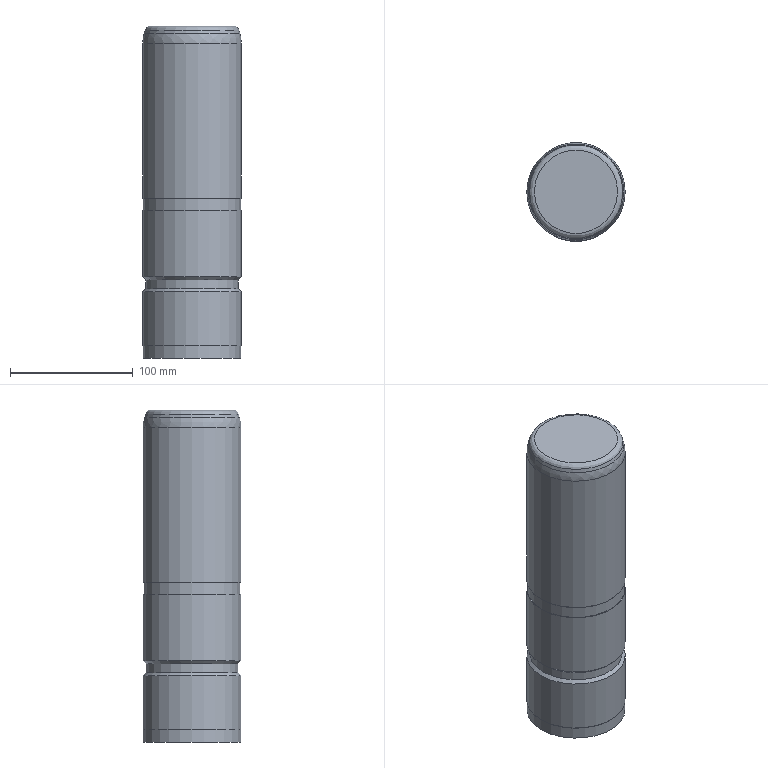Part | NX | features solid 2 | 1 solid | 16 faces | box 80 x 80 x 270 mm | volume 1345505 mm3 | cylinder 6 | plane 5 | cone 3 | torus 2 | commonest cylinder face diameters 80 x3 75 x1 79 x1 79.5 x1
STEP:
#1=CARTESIAN_POINT('',(-1152.5,955.,-291.5));
#2=VERTEX_POINT('',#1);
#3=CARTESIAN_POINT('',(-1115.,955.,-291.5));
#4=DIRECTION('',(0.,0.,1.));
#5=DIRECTION('',(-1.,0.,0.));
#6=AXIS2_PLACEMENT_3D('',#3,#4,#5);
#7=CIRCLE('',#6,37.5);
#8=EDGE_CURVE('',#2,#2,#7,.T.);
#9=ORIENTED_EDGE('',*,*,#8,.T.);
#10=EDGE_LOOP('',(#9));
#11=FACE_BOUND('',#10,.T.);
#12=CARTESIAN_POINT('',(-1075.,955.,-289.));
#13=VERTEX_POINT('',#12);
#14=CARTESIAN_POINT('',(-1115.,955.,-289.));
#15=DIRECTION('',(0.,0.,-1.));
#16=DIRECTION('',(1.,0.,0.));
#17=AXIS2_PLACEMENT_3D('',#14,#15,#16);
#18=CIRCLE('',#17,40.);
#19=EDGE_CURVE('',#13,#13,#18,.T.);
#20=ORIENTED_EDGE('',*,*,#19,.T.);
#21=EDGE_LOOP('',(#20));
#22=FACE_BOUND('',#21,.T.);
#23=CARTESIAN_POINT('',(-1115.,955.,-291.5));
#24=DIRECTION('',(0.,0.,1.));
#25=DIRECTION('',(1.,0.,0.));
#26=AXIS2_PLACEMENT_3D('',#23,#24,#25);
#27=CONICAL_SURFACE('',#26,37.5,0.7854);
#28=ADVANCED_FACE('',(#11,#22),#27,.T.);
#29=ORIENTED_EDGE('',*,*,#8,.F.);
#30=EDGE_LOOP('',(#29));
#31=FACE_BOUND('',#30,.T.);
#32=CARTESIAN_POINT('',(-1152.5,955.,-298.5));
#33=VERTEX_POINT('',#32);
#34=CARTESIAN_POINT('',(-1115.,955.,-298.5));
#35=DIRECTION('',(0.,0.,1.));
#36=DIRECTION('',(-1.,0.,0.));
#37=AXIS2_PLACEMENT_3D('',#34,#35,#36);
#38=CIRCLE('',#37,37.5);
#39=EDGE_CURVE('',#33,#33,#38,.T.);
#40=ORIENTED_EDGE('',*,*,#39,.T.);
#41=EDGE_LOOP('',(#40));
#42=FACE_BOUND('',#41,.T.);
#43=CARTESIAN_POINT('',(-1115.,955.,-298.5));
#44=DIRECTION('',(0.,0.,1.));
#45=DIRECTION('',(1.,0.,0.));
#46=AXIS2_PLACEMENT_3D('',#43,#44,#45);
#47=CYLINDRICAL_SURFACE('',#46,37.5);
#48=ADVANCED_FACE('',(#31,#42),#47,.T.);
#49=CARTESIAN_POINT('',(-1075.5,955.,-235.));
#50=VERTEX_POINT('',#49);
#51=CARTESIAN_POINT('',(-1115.,955.,-235.));
#52=DIRECTION('',(0.,0.,-1.));
#53=DIRECTION('',(1.,0.,0.));
#54=AXIS2_PLACEMENT_3D('',#51,#52,#53);
#55=CIRCLE('',#54,39.5);
#56=EDGE_CURVE('',#50,#50,#55,.T.);
#57=ORIENTED_EDGE('',*,*,#56,.T.);
#58=EDGE_LOOP('',(#57));
#59=FACE_BOUND('',#58,.T.);
#60=CARTESIAN_POINT('',(-1155.,955.,-235.));
#61=VERTEX_POINT('',#60);
#62=CARTESIAN_POINT('',(-1115.,955.,-235.));
#63=DIRECTION('',(0.,0.,1.));
#64=DIRECTION('',(-1.,0.,0.));
#65=AXIS2_PLACEMENT_3D('',#62,#63,#64);
#66=CIRCLE('',#65,40.);
#67=EDGE_CURVE('',#61,#61,#66,.T.);
#68=ORIENTED_EDGE('',*,*,#67,.T.);
#69=EDGE_LOOP('',(#68));
#70=FACE_BOUND('',#69,.T.);
#71=CARTESIAN_POINT('',(-1115.,955.,-235.));
#72=DIRECTION('',(0.,0.,1.));
#73=DIRECTION('',(1.,0.,0.));
#74=AXIS2_PLACEMENT_3D('',#71,#72,#73);
#75=PLANE('',#74);
#76=ADVANCED_FACE('',(#59,#70),#75,.T.);
#77=ORIENTED_EDGE('',*,*,#67,.F.);
#78=EDGE_LOOP('',(#77));
#79=FACE_BOUND('',#78,.T.);
#80=ORIENTED_EDGE('',*,*,#19,.F.);
#81=EDGE_LOOP('',(#80));
#82=FACE_BOUND('',#81,.T.);
#83=CARTESIAN_POINT('',(-1115.,955.,-289.));
#84=DIRECTION('',(0.,0.,1.));
#85=DIRECTION('',(1.,0.,0.));
#86=AXIS2_PLACEMENT_3D('',#83,#84,#85);
#87=CYLINDRICAL_SURFACE('',#86,40.);
#88=ADVANCED_FACE('',(#79,#82),#87,.T.);
#89=CARTESIAN_POINT('',(-1154.5,955.,-225.));
#90=VERTEX_POINT('',#89);
#91=CARTESIAN_POINT('',(-1115.,955.,-225.));
#92=DIRECTION('',(0.,0.,-1.));
#93=DIRECTION('',(-1.,0.,0.));
#94=AXIS2_PLACEMENT_3D('',#91,#92,#93);
#95=CIRCLE('',#94,39.5);
#96=EDGE_CURVE('',#90,#90,#95,.F.);
#97=ORIENTED_EDGE('',*,*,#96,.F.);
#98=EDGE_LOOP('',(#97));
#99=FACE_BOUND('',#98,.T.);
#100=ORIENTED_EDGE('',*,*,#56,.F.);
#101=EDGE_LOOP('',(#100));
#102=FACE_BOUND('',#101,.T.);
#103=CARTESIAN_POINT('',(-1115.,955.,-235.));
#104=DIRECTION('',(0.,0.,1.));
#105=DIRECTION('',(1.,0.,0.));
#106=AXIS2_PLACEMENT_3D('',#103,#104,#105);
#107=CYLINDRICAL_SURFACE('',#106,39.5);
#108=ADVANCED_FACE('',(#99,#102),#107,.T.);
#109=CARTESIAN_POINT('',(-1154.75,955.,-345.));
#110=VERTEX_POINT('',#109);
#111=CARTESIAN_POINT('',(-1115.,955.,-345.));
#112=DIRECTION('',(0.,0.,1.));
#113=DIRECTION('',(-1.,0.,0.));
#114=AXIS2_PLACEMENT_3D('',#111,#112,#113);
#115=CIRCLE('',#114,39.75);
#116=EDGE_CURVE('',#110,#110,#115,.T.);
#117=ORIENTED_EDGE('',*,*,#116,.T.);
#118=EDGE_LOOP('',(#117));
#119=FACE_BOUND('',#118,.T.);
#120=CARTESIAN_POINT('',(-1075.,955.,-345.));
#121=VERTEX_POINT('',#120);
#122=CARTESIAN_POINT('',(-1115.,955.,-345.));
#123=DIRECTION('',(0.,0.,-1.));
#124=DIRECTION('',(1.,0.,0.));
#125=AXIS2_PLACEMENT_3D('',#122,#123,#124);
#126=CIRCLE('',#125,40.);
#127=EDGE_CURVE('',#121,#121,#126,.T.);
#128=ORIENTED_EDGE('',*,*,#127,.T.);
#129=EDGE_LOOP('',(#128));
#130=FACE_BOUND('',#129,.T.);
#131=CARTESIAN_POINT('',(-1115.,955.,-345.));
#132=DIRECTION('',(0.,0.,-1.));
#133=DIRECTION('',(-1.,0.,0.));
#134=AXIS2_PLACEMENT_3D('',#131,#132,#133);
#135=PLANE('',#134);
#136=ADVANCED_FACE('',(#119,#130),#135,.T.);
#137=CARTESIAN_POINT('',(-1075.,955.,-301.));
#138=VERTEX_POINT('',#137);
#139=CARTESIAN_POINT('',(-1115.,955.,-301.));
#140=DIRECTION('',(0.,0.,-1.));
#141=DIRECTION('',(1.,0.,0.));
#142=AXIS2_PLACEMENT_3D('',#139,#140,#141);
#143=CIRCLE('',#142,40.);
#144=EDGE_CURVE('',#138,#138,#143,.T.);
#145=ORIENTED_EDGE('',*,*,#144,.T.);
#146=EDGE_LOOP('',(#145));
#147=FACE_BOUND('',#146,.T.);
#148=ORIENTED_EDGE('',*,*,#127,.F.);
#149=EDGE_LOOP('',(#148));
#150=FACE_BOUND('',#149,.T.);
#151=CARTESIAN_POINT('',(-1115.,955.,-345.));
#152=DIRECTION('',(0.,0.,1.));
#153=DIRECTION('',(1.,0.,0.));
#154=AXIS2_PLACEMENT_3D('',#151,#152,#153);
#155=CYLINDRICAL_SURFACE('',#154,40.);
#156=ADVANCED_FACE('',(#147,#150),#155,.T.);
#157=CARTESIAN_POINT('',(-1075.25,955.,-355.));
#158=VERTEX_POINT('',#157);
#159=CARTESIAN_POINT('',(-1115.,955.,-355.));
#160=DIRECTION('',(0.,0.,-1.));
#161=DIRECTION('',(1.,0.,0.));
#162=AXIS2_PLACEMENT_3D('',#159,#160,#161);
#163=CIRCLE('',#162,39.75);
#164=EDGE_CURVE('',#158,#158,#163,.T.);
#165=ORIENTED_EDGE('',*,*,#164,.T.);
#166=EDGE_LOOP('',(#165));
#167=FACE_BOUND('',#166,.T.);
#168=CARTESIAN_POINT('',(-1115.,955.,-355.));
#169=DIRECTION('',(0.,0.,-1.));
#170=DIRECTION('',(-1.,0.,0.));
#171=AXIS2_PLACEMENT_3D('',#168,#169,#170);
#172=PLANE('',#171);
#173=ADVANCED_FACE('',(#167),#172,.T.);
#174=ORIENTED_EDGE('',*,*,#116,.F.);
#175=EDGE_LOOP('',(#174));
#176=FACE_BOUND('',#175,.T.);
#177=ORIENTED_EDGE('',*,*,#164,.F.);
#178=EDGE_LOOP('',(#177));
#179=FACE_BOUND('',#178,.T.);
#180=CARTESIAN_POINT('',(-1115.,955.,-355.));
#181=DIRECTION('',(0.,0.,1.));
#182=DIRECTION('',(1.,0.,0.));
#183=AXIS2_PLACEMENT_3D('',#180,#181,#182);
#184=CYLINDRICAL_SURFACE('',#183,39.75);
#185=ADVANCED_FACE('',(#176,#179),#184,.T.);
#186=ORIENTED_EDGE('',*,*,#144,.F.);
#187=EDGE_LOOP('',(#186));
#188=FACE_BOUND('',#187,.T.);
#189=ORIENTED_EDGE('',*,*,#39,.F.);
#190=EDGE_LOOP('',(#189));
#191=FACE_BOUND('',#190,.T.);
#192=CARTESIAN_POINT('',(-1115.,955.,-298.5));
#193=DIRECTION('',(0.,0.,-1.));
#194=DIRECTION('',(-1.,0.,0.));
#195=AXIS2_PLACEMENT_3D('',#192,#193,#194);
#196=CONICAL_SURFACE('',#195,37.5,0.7854);
#197=ADVANCED_FACE('',(#188,#191),#196,.T.);
#198=CARTESIAN_POINT('',(-1081.132,955.,-85.));
#199=VERTEX_POINT('',#198);
#200=CARTESIAN_POINT('',(-1115.,955.,-85.));
#201=DIRECTION('',(0.,0.,-1.));
#202=DIRECTION('',(1.,0.,0.));
#203=AXIS2_PLACEMENT_3D('',#200,#201,#202);
#204=CIRCLE('',#203,33.868);
#205=EDGE_CURVE('',#199,#199,#204,.T.);
#206=ORIENTED_EDGE('',*,*,#205,.F.);
#207=EDGE_LOOP('',(#206));
#208=FACE_BOUND('',#207,.T.);
#209=CARTESIAN_POINT('',(-1115.,955.,-85.));
#210=DIRECTION('',(0.,0.,1.));
#211=DIRECTION('',(1.,0.,0.));
#212=AXIS2_PLACEMENT_3D('',#209,#210,#211);
#213=PLANE('',#212);
#214=ADVANCED_FACE('',(#208),#213,.T.);
#215=ORIENTED_EDGE('',*,*,#205,.T.);
#216=EDGE_LOOP('',(#215));
#217=FACE_BOUND('',#216,.T.);
#218=CARTESIAN_POINT('',(-1076.786,955.,-88.335));
#219=VERTEX_POINT('',#218);
#220=CARTESIAN_POINT('',(-1115.,955.,-88.335));
#221=DIRECTION('',(0.,0.,-1.));
#222=DIRECTION('',(1.,0.,0.));
#223=AXIS2_PLACEMENT_3D('',#220,#221,#222);
#224=CIRCLE('',#223,38.214);
#225=EDGE_CURVE('',#219,#219,#224,.F.);
#226=ORIENTED_EDGE('',*,*,#225,.T.);
#227=EDGE_LOOP('',(#226));
#228=FACE_BOUND('',#227,.T.);
#229=CARTESIAN_POINT('',(-1115.,955.,-89.5));
#230=DIRECTION('',(0.,0.,1.));
#231=DIRECTION('',(1.,0.,0.));
#232=AXIS2_PLACEMENT_3D('',#229,#230,#231);
#233=TOROIDAL_SURFACE('',#232,33.868,4.5);
#234=ADVANCED_FACE('',(#217,#228),#233,.T.);
#235=ORIENTED_EDGE('',*,*,#225,.F.);
#236=EDGE_LOOP('',(#235));
#237=FACE_BOUND('',#236,.T.);
#238=CARTESIAN_POINT('',(-1076.022,955.,-91.185));
#239=VERTEX_POINT('',#238);
#240=CARTESIAN_POINT('',(-1115.,955.,-91.185));
#241=DIRECTION('',(0.,0.,-1.));
#242=DIRECTION('',(1.,0.,0.));
#243=AXIS2_PLACEMENT_3D('',#240,#241,#242);
#244=CIRCLE('',#243,38.978);
#245=EDGE_CURVE('',#239,#239,#244,.T.);
#246=ORIENTED_EDGE('',*,*,#245,.F.);
#247=EDGE_LOOP('',(#246));
#248=FACE_BOUND('',#247,.T.);
#249=CARTESIAN_POINT('',(-1115.,955.,-85.));
#250=DIRECTION('',(0.,0.,-1.));
#251=DIRECTION('',(-1.,0.,0.));
#252=AXIS2_PLACEMENT_3D('',#249,#250,#251);
#253=CONICAL_SURFACE('',#252,37.321,0.2618);
#254=ADVANCED_FACE('',(#237,#248),#253,.T.);
#255=CARTESIAN_POINT('',(-1155.,955.,-98.95));
#256=VERTEX_POINT('',#255);
#257=CARTESIAN_POINT('',(-1115.,955.,-98.95));
#258=DIRECTION('',(0.,0.,1.));
#259=DIRECTION('',(-1.,0.,0.));
#260=AXIS2_PLACEMENT_3D('',#257,#258,#259);
#261=CIRCLE('',#260,40.);
#262=EDGE_CURVE('',#256,#256,#261,.T.);
#263=ORIENTED_EDGE('',*,*,#262,.T.);
#264=EDGE_LOOP('',(#263));
#265=FACE_BOUND('',#264,.T.);
#266=ORIENTED_EDGE('',*,*,#245,.T.);
#267=EDGE_LOOP('',(#266));
#268=FACE_BOUND('',#267,.T.);
#269=CARTESIAN_POINT('',(-1115.,955.,-98.95));
#270=DIRECTION('',(0.,0.,-1.));
#271=DIRECTION('',(-1.,0.,0.));
#272=AXIS2_PLACEMENT_3D('',#269,#270,#271);
#273=DEGENERATE_TOROIDAL_SURFACE('',#272,10.,30.,.T.);
#274=ADVANCED_FACE('',(#265,#268),#273,.T.);
#275=ORIENTED_EDGE('',*,*,#262,.F.);
#276=EDGE_LOOP('',(#275));
#277=FACE_BOUND('',#276,.T.);
#278=CARTESIAN_POINT('',(-1155.,955.,-225.));
#279=VERTEX_POINT('',#278);
#280=CARTESIAN_POINT('',(-1115.,955.,-225.));
#281=DIRECTION('',(0.,0.,-1.));
#282=DIRECTION('',(-1.,0.,0.));
#283=AXIS2_PLACEMENT_3D('',#280,#281,#282);
#284=CIRCLE('',#283,40.);
#285=EDGE_CURVE('',#279,#279,#284,.T.);
#286=ORIENTED_EDGE('',*,*,#285,.F.);
#287=EDGE_LOOP('',(#286));
#288=FACE_BOUND('',#287,.T.);
#289=CARTESIAN_POINT('',(-1115.,955.,-205.));
#290=DIRECTION('',(0.,0.,1.));
#291=DIRECTION('',(1.,0.,0.));
#292=AXIS2_PLACEMENT_3D('',#289,#290,#291);
#293=CYLINDRICAL_SURFACE('',#292,40.);
#294=ADVANCED_FACE('',(#277,#288),#293,.T.);
#295=ORIENTED_EDGE('',*,*,#96,.T.);
#296=EDGE_LOOP('',(#295));
#297=FACE_BOUND('',#296,.T.);
#298=ORIENTED_EDGE('',*,*,#285,.T.);
#299=EDGE_LOOP('',(#298));
#300=FACE_BOUND('',#299,.T.);
#301=CARTESIAN_POINT('',(-1115.,955.,-225.));
#302=DIRECTION('',(0.,0.,-1.));
#303=DIRECTION('',(-1.,0.,0.));
#304=AXIS2_PLACEMENT_3D('',#301,#302,#303);
#305=PLANE('',#304);
#306=ADVANCED_FACE('',(#297,#300),#305,.T.);
#307=CLOSED_SHELL('',(#28,#48,#76,#88,#108,#136,#156,#173,#185,#197,#214,#234,#254,#274,#294,#306));
#308=MANIFOLD_SOLID_BREP('',#307);
#309=(LENGTH_UNIT()NAMED_UNIT(*)SI_UNIT(.MILLI.,.METRE.));
#310=UNCERTAINTY_MEASURE_WITH_UNIT(LENGTH_MEASURE(0.00001),#309,'','');
#311=(NAMED_UNIT(*)PLANE_ANGLE_UNIT()SI_UNIT($,.RADIAN.));
#312=(NAMED_UNIT(*)SI_UNIT($,.STERADIAN.)SOLID_ANGLE_UNIT());
#313=(GEOMETRIC_REPRESENTATION_CONTEXT(3)GLOBAL_UNCERTAINTY_ASSIGNED_CONTEXT((#310))GLOBAL_UNIT_ASSIGNED_CONTEXT((#309,#311,#312))REPRESENTATION_CONTEXT('',''));
#314=ADVANCED_BREP_SHAPE_REPRESENTATION('',(#308),#313);